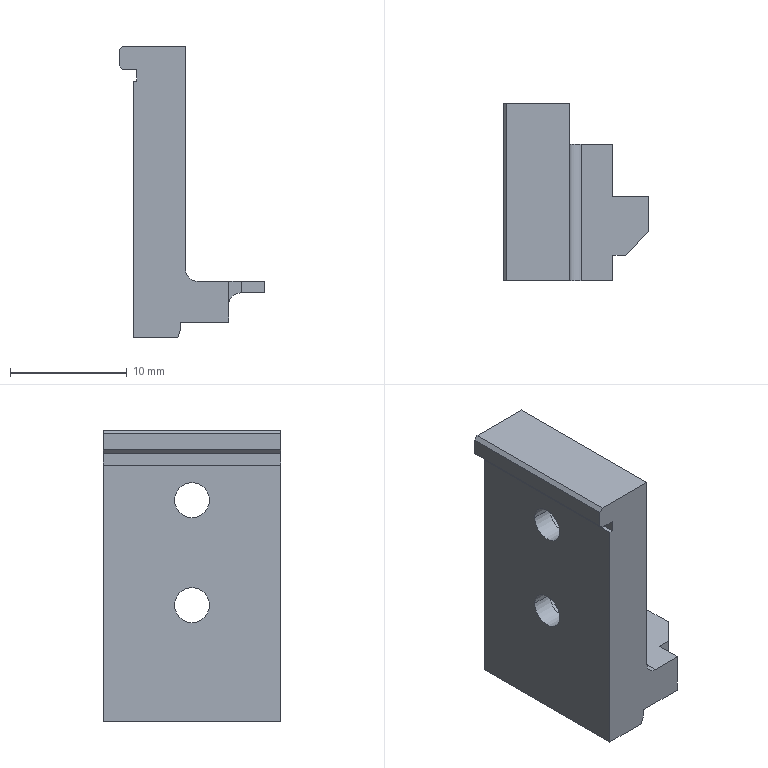Part | NX | 1 solid | 35 faces | box 12.5 x 15.2 x 25 mm | volume 1768 mm3 | plane 25 | cylinder 10 | commonest cylinder face diameters 3 x4 5 x4 2 x2
STEP:
#1=CARTESIAN_POINT('',(-1.77,0.,-1.43));
#2=VERTEX_POINT('',#1);
#3=CARTESIAN_POINT('',(-2.025,0.,-2.13));
#4=VERTEX_POINT('',#3);
#5=CARTESIAN_POINT('',(-1.25,0.,0.));
#6=DIRECTION('',(-0.342,0.,-0.9397));
#7=VECTOR('',#6,1000.);
#8=LINE('',#5,#7);
#9=EDGE_CURVE('',#2,#4,#8,.T.);
#10=ORIENTED_EDGE('',*,*,#9,.T.);
#11=CARTESIAN_POINT('',(-5.85,0.,-2.13));
#12=VERTEX_POINT('',#11);
#13=CARTESIAN_POINT('',(0.,0.,-2.13));
#14=DIRECTION('',(1.,0.,0.));
#15=VECTOR('',#14,1000.);
#16=LINE('',#13,#15);
#17=EDGE_CURVE('',#12,#4,#16,.T.);
#18=ORIENTED_EDGE('',*,*,#17,.F.);
#19=CARTESIAN_POINT('',(-5.85,0.,19.87));
#20=VERTEX_POINT('',#19);
#21=CARTESIAN_POINT('',(-5.85,0.,0.));
#22=DIRECTION('',(0.,0.,1.));
#23=VECTOR('',#22,1000.);
#24=LINE('',#21,#23);
#25=EDGE_CURVE('',#12,#20,#24,.T.);
#26=ORIENTED_EDGE('',*,*,#25,.T.);
#27=CARTESIAN_POINT('',(-5.55,0.,19.87));
#28=VERTEX_POINT('',#27);
#29=CARTESIAN_POINT('',(0.,0.,19.87));
#30=DIRECTION('',(1.,0.,0.));
#31=VECTOR('',#30,1000.);
#32=LINE('',#29,#31);
#33=EDGE_CURVE('',#20,#28,#32,.T.);
#34=ORIENTED_EDGE('',*,*,#33,.T.);
#35=CARTESIAN_POINT('',(-5.55,0.,20.87));
#36=VERTEX_POINT('',#35);
#37=CARTESIAN_POINT('',(-5.55,0.,0.));
#38=DIRECTION('',(0.,0.,1.));
#39=VECTOR('',#38,1000.);
#40=LINE('',#37,#39);
#41=EDGE_CURVE('',#28,#36,#40,.T.);
#42=ORIENTED_EDGE('',*,*,#41,.T.);
#43=CARTESIAN_POINT('',(-6.75,0.,20.87));
#44=VERTEX_POINT('',#43);
#45=CARTESIAN_POINT('',(0.,0.,20.87));
#46=DIRECTION('',(-1.,0.,0.));
#47=VECTOR('',#46,1000.);
#48=LINE('',#45,#47);
#49=EDGE_CURVE('',#36,#44,#48,.T.);
#50=ORIENTED_EDGE('',*,*,#49,.T.);
#51=CARTESIAN_POINT('',(-7.05,0.,21.17));
#52=VERTEX_POINT('',#51);
#53=CARTESIAN_POINT('',(14.12,0.,0.));
#54=DIRECTION('',(0.7071,0.,-0.7071));
#55=VECTOR('',#54,1000.);
#56=LINE('',#53,#55);
#57=EDGE_CURVE('',#52,#44,#56,.T.);
#58=ORIENTED_EDGE('',*,*,#57,.F.);
#59=CARTESIAN_POINT('',(-7.05,0.,22.57));
#60=VERTEX_POINT('',#59);
#61=CARTESIAN_POINT('',(-7.05,0.,0.));
#62=DIRECTION('',(0.,0.,1.));
#63=VECTOR('',#62,1000.);
#64=LINE('',#61,#63);
#65=EDGE_CURVE('',#52,#60,#64,.T.);
#66=ORIENTED_EDGE('',*,*,#65,.T.);
#67=CARTESIAN_POINT('',(-6.75,0.,22.87));
#68=VERTEX_POINT('',#67);
#69=CARTESIAN_POINT('',(-29.62,0.,0.));
#70=DIRECTION('',(0.7071,0.,0.7071));
#71=VECTOR('',#70,1000.);
#72=LINE('',#69,#71);
#73=EDGE_CURVE('',#60,#68,#72,.T.);
#74=ORIENTED_EDGE('',*,*,#73,.T.);
#75=CARTESIAN_POINT('',(-1.35,0.,22.87));
#76=VERTEX_POINT('',#75);
#77=CARTESIAN_POINT('',(0.,0.,22.87));
#78=DIRECTION('',(1.,0.,0.));
#79=VECTOR('',#78,1000.);
#80=LINE('',#77,#79);
#81=EDGE_CURVE('',#68,#76,#80,.T.);
#82=ORIENTED_EDGE('',*,*,#81,.T.);
#83=CARTESIAN_POINT('',(-1.35,0.,-0.78));
#84=VERTEX_POINT('',#83);
#85=CARTESIAN_POINT('',(-1.35,0.,0.));
#86=DIRECTION('',(0.,0.,1.));
#87=VECTOR('',#86,1000.);
#88=LINE('',#85,#87);
#89=EDGE_CURVE('',#84,#76,#88,.T.);
#90=ORIENTED_EDGE('',*,*,#89,.F.);
#91=CARTESIAN_POINT('',(-1.77,0.,-0.78));
#92=VERTEX_POINT('',#91);
#93=CARTESIAN_POINT('',(0.,0.,-0.78));
#94=DIRECTION('',(-1.,0.,0.));
#95=VECTOR('',#94,1000.);
#96=LINE('',#93,#95);
#97=EDGE_CURVE('',#84,#92,#96,.T.);
#98=ORIENTED_EDGE('',*,*,#97,.T.);
#99=CARTESIAN_POINT('',(-1.77,0.,0.));
#100=DIRECTION('',(0.,0.,-1.));
#101=VECTOR('',#100,1000.);
#102=LINE('',#99,#101);
#103=EDGE_CURVE('',#92,#2,#102,.T.);
#104=ORIENTED_EDGE('',*,*,#103,.T.);
#105=EDGE_LOOP('',(#10,#18,#26,#34,#42,#50,#58,#66,#74,#82,#90,#98,#104));
#106=FACE_BOUND('',#105,.T.);
#107=CARTESIAN_POINT('',(0.,0.,0.));
#108=DIRECTION('',(0.,-1.,0.));
#109=DIRECTION('',(0.,0.,-1.));
#110=AXIS2_PLACEMENT_3D('',#107,#108,#109);
#111=PLANE('',#110);
#112=ADVANCED_FACE('',(#106),#111,.F.);
#113=CARTESIAN_POINT('',(-1.77,-15.2,-1.43));
#114=VERTEX_POINT('',#113);
#115=CARTESIAN_POINT('',(-1.77,0.,-1.43));
#116=DIRECTION('',(0.,-1.,0.));
#117=VECTOR('',#116,1000.);
#118=LINE('',#115,#117);
#119=EDGE_CURVE('',#2,#114,#118,.T.);
#120=ORIENTED_EDGE('',*,*,#119,.F.);
#121=ORIENTED_EDGE('',*,*,#103,.F.);
#122=CARTESIAN_POINT('',(-1.77,-15.2,-0.78));
#123=VERTEX_POINT('',#122);
#124=CARTESIAN_POINT('',(-1.77,0.,-0.78));
#125=DIRECTION('',(0.,1.,0.));
#126=VECTOR('',#125,1000.);
#127=LINE('',#124,#126);
#128=EDGE_CURVE('',#123,#92,#127,.T.);
#129=ORIENTED_EDGE('',*,*,#128,.F.);
#130=CARTESIAN_POINT('',(-1.77,-15.2,0.));
#131=DIRECTION('',(0.,0.,1.));
#132=VECTOR('',#131,1000.);
#133=LINE('',#130,#132);
#134=EDGE_CURVE('',#114,#123,#133,.T.);
#135=ORIENTED_EDGE('',*,*,#134,.F.);
#136=EDGE_LOOP('',(#120,#121,#129,#135));
#137=FACE_BOUND('',#136,.T.);
#138=CARTESIAN_POINT('',(-1.77,0.,-0.93));
#139=DIRECTION('',(1.,0.,0.));
#140=DIRECTION('',(0.,1.,0.));
#141=AXIS2_PLACEMENT_3D('',#138,#139,#140);
#142=PLANE('',#141);
#143=ADVANCED_FACE('',(#137),#142,.T.);
#144=CARTESIAN_POINT('',(-0.35,-15.2,2.72));
#145=VERTEX_POINT('',#144);
#146=CARTESIAN_POINT('',(2.35,-15.2,2.72));
#147=VERTEX_POINT('',#146);
#148=CARTESIAN_POINT('',(0.,-15.2,2.72));
#149=DIRECTION('',(1.,0.,0.));
#150=VECTOR('',#149,1000.);
#151=LINE('',#148,#150);
#152=EDGE_CURVE('',#145,#147,#151,.T.);
#153=ORIENTED_EDGE('',*,*,#152,.F.);
#154=CARTESIAN_POINT('',(-1.35,-15.2,3.72));
#155=VERTEX_POINT('',#154);
#156=CARTESIAN_POINT('',(-0.35,-15.2,3.72));
#157=DIRECTION('',(0.,1.,0.));
#158=DIRECTION('',(-1.,0.,0.));
#159=AXIS2_PLACEMENT_3D('',#156,#157,#158);
#160=CIRCLE('',#159,1.);
#161=EDGE_CURVE('',#145,#155,#160,.T.);
#162=ORIENTED_EDGE('',*,*,#161,.T.);
#163=CARTESIAN_POINT('',(-1.35,-15.2,22.87));
#164=VERTEX_POINT('',#163);
#165=CARTESIAN_POINT('',(-1.35,-15.2,0.));
#166=DIRECTION('',(0.,0.,-1.));
#167=VECTOR('',#166,1000.);
#168=LINE('',#165,#167);
#169=EDGE_CURVE('',#164,#155,#168,.T.);
#170=ORIENTED_EDGE('',*,*,#169,.F.);
#171=CARTESIAN_POINT('',(-6.75,-15.2,22.87));
#172=VERTEX_POINT('',#171);
#173=CARTESIAN_POINT('',(0.,-15.2,22.87));
#174=DIRECTION('',(-1.,0.,0.));
#175=VECTOR('',#174,1000.);
#176=LINE('',#173,#175);
#177=EDGE_CURVE('',#164,#172,#176,.T.);
#178=ORIENTED_EDGE('',*,*,#177,.T.);
#179=CARTESIAN_POINT('',(-7.05,-15.2,22.57));
#180=VERTEX_POINT('',#179);
#181=CARTESIAN_POINT('',(-29.62,-15.2,0.));
#182=DIRECTION('',(-0.7071,0.,-0.7071));
#183=VECTOR('',#182,1000.);
#184=LINE('',#181,#183);
#185=EDGE_CURVE('',#172,#180,#184,.T.);
#186=ORIENTED_EDGE('',*,*,#185,.T.);
#187=CARTESIAN_POINT('',(-7.05,-15.2,21.17));
#188=VERTEX_POINT('',#187);
#189=CARTESIAN_POINT('',(-7.05,-15.2,0.));
#190=DIRECTION('',(0.,0.,-1.));
#191=VECTOR('',#190,1000.);
#192=LINE('',#189,#191);
#193=EDGE_CURVE('',#180,#188,#192,.T.);
#194=ORIENTED_EDGE('',*,*,#193,.T.);
#195=CARTESIAN_POINT('',(-6.75,-15.2,20.87));
#196=VERTEX_POINT('',#195);
#197=CARTESIAN_POINT('',(14.12,-15.2,0.));
#198=DIRECTION('',(-0.7071,0.,0.7071));
#199=VECTOR('',#198,1000.);
#200=LINE('',#197,#199);
#201=EDGE_CURVE('',#196,#188,#200,.T.);
#202=ORIENTED_EDGE('',*,*,#201,.F.);
#203=CARTESIAN_POINT('',(-5.55,-15.2,20.87));
#204=VERTEX_POINT('',#203);
#205=CARTESIAN_POINT('',(0.,-15.2,20.87));
#206=DIRECTION('',(1.,0.,0.));
#207=VECTOR('',#206,1000.);
#208=LINE('',#205,#207);
#209=EDGE_CURVE('',#196,#204,#208,.T.);
#210=ORIENTED_EDGE('',*,*,#209,.T.);
#211=CARTESIAN_POINT('',(-5.55,-15.2,19.87));
#212=VERTEX_POINT('',#211);
#213=CARTESIAN_POINT('',(-5.55,-15.2,0.));
#214=DIRECTION('',(0.,0.,-1.));
#215=VECTOR('',#214,1000.);
#216=LINE('',#213,#215);
#217=EDGE_CURVE('',#204,#212,#216,.T.);
#218=ORIENTED_EDGE('',*,*,#217,.T.);
#219=CARTESIAN_POINT('',(-5.85,-15.2,19.87));
#220=VERTEX_POINT('',#219);
#221=CARTESIAN_POINT('',(0.,-15.2,19.87));
#222=DIRECTION('',(-1.,0.,0.));
#223=VECTOR('',#222,1000.);
#224=LINE('',#221,#223);
#225=EDGE_CURVE('',#212,#220,#224,.T.);
#226=ORIENTED_EDGE('',*,*,#225,.T.);
#227=CARTESIAN_POINT('',(-5.85,-15.2,-2.13));
#228=VERTEX_POINT('',#227);
#229=CARTESIAN_POINT('',(-5.85,-15.2,0.));
#230=DIRECTION('',(0.,0.,-1.));
#231=VECTOR('',#230,1000.);
#232=LINE('',#229,#231);
#233=EDGE_CURVE('',#220,#228,#232,.T.);
#234=ORIENTED_EDGE('',*,*,#233,.T.);
#235=CARTESIAN_POINT('',(-2.025,-15.2,-2.13));
#236=VERTEX_POINT('',#235);
#237=CARTESIAN_POINT('',(0.,-15.2,-2.13));
#238=DIRECTION('',(-1.,0.,0.));
#239=VECTOR('',#238,1000.);
#240=LINE('',#237,#239);
#241=EDGE_CURVE('',#236,#228,#240,.T.);
#242=ORIENTED_EDGE('',*,*,#241,.F.);
#243=CARTESIAN_POINT('',(-1.25,-15.2,0.));
#244=DIRECTION('',(0.342,0.,0.9397));
#245=VECTOR('',#244,1000.);
#246=LINE('',#243,#245);
#247=EDGE_CURVE('',#236,#114,#246,.T.);
#248=ORIENTED_EDGE('',*,*,#247,.T.);
#249=ORIENTED_EDGE('',*,*,#134,.T.);
#250=CARTESIAN_POINT('',(2.35,-15.2,-0.78));
#251=VERTEX_POINT('',#250);
#252=CARTESIAN_POINT('',(0.,-15.2,-0.78));
#253=DIRECTION('',(1.,0.,0.));
#254=VECTOR('',#253,1000.);
#255=LINE('',#252,#254);
#256=EDGE_CURVE('',#123,#251,#255,.T.);
#257=ORIENTED_EDGE('',*,*,#256,.T.);
#258=CARTESIAN_POINT('',(2.35,-15.2,0.));
#259=DIRECTION('',(0.,0.,1.));
#260=VECTOR('',#259,1000.);
#261=LINE('',#258,#260);
#262=EDGE_CURVE('',#251,#147,#261,.T.);
#263=ORIENTED_EDGE('',*,*,#262,.T.);
#264=EDGE_LOOP('',(#153,#162,#170,#178,#186,#194,#202,#210,#218,#226,#234,#242,#248,#249,#257,#263));
#265=FACE_BOUND('',#264,.T.);
#266=CARTESIAN_POINT('',(-1.35,-15.2,0.));
#267=DIRECTION('',(0.,1.,0.));
#268=DIRECTION('',(1.,0.,0.));
#269=AXIS2_PLACEMENT_3D('',#266,#267,#268);
#270=PLANE('',#269);
#271=ADVANCED_FACE('',(#265),#270,.F.);
#272=CARTESIAN_POINT('',(-4.05,-10.1,7.87));
#273=VERTEX_POINT('',#272);
#274=CARTESIAN_POINT('',(-4.05,-5.1,7.87));
#275=VERTEX_POINT('',#274);
#276=CARTESIAN_POINT('',(-4.05,-7.6,7.87));
#277=DIRECTION('',(1.,0.,0.));
#278=DIRECTION('',(0.,-1.,0.));
#279=AXIS2_PLACEMENT_3D('',#276,#277,#278);
#280=CIRCLE('',#279,2.5);
#281=EDGE_CURVE('',#273,#275,#280,.T.);
#282=ORIENTED_EDGE('',*,*,#281,.T.);
#283=CARTESIAN_POINT('',(-4.05,-7.6,7.87));
#284=DIRECTION('',(1.,0.,0.));
#285=DIRECTION('',(0.,-1.,0.));
#286=AXIS2_PLACEMENT_3D('',#283,#284,#285);
#287=CIRCLE('',#286,2.5);
#288=EDGE_CURVE('',#275,#273,#287,.T.);
#289=ORIENTED_EDGE('',*,*,#288,.T.);
#290=EDGE_LOOP('',(#282,#289));
#291=FACE_BOUND('',#290,.T.);
#292=CARTESIAN_POINT('',(-4.05,-6.1,7.87));
#293=VERTEX_POINT('',#292);
#294=CARTESIAN_POINT('',(-4.05,-9.1,7.87));
#295=VERTEX_POINT('',#294);
#296=CARTESIAN_POINT('',(-4.05,-7.6,7.87));
#297=DIRECTION('',(1.,0.,0.));
#298=DIRECTION('',(0.,-1.,0.));
#299=AXIS2_PLACEMENT_3D('',#296,#297,#298);
#300=CIRCLE('',#299,1.5);
#301=EDGE_CURVE('',#293,#295,#300,.T.);
#302=ORIENTED_EDGE('',*,*,#301,.F.);
#303=CARTESIAN_POINT('',(-4.05,-7.6,7.87));
#304=DIRECTION('',(1.,0.,0.));
#305=DIRECTION('',(0.,-1.,0.));
#306=AXIS2_PLACEMENT_3D('',#303,#304,#305);
#307=CIRCLE('',#306,1.5);
#308=EDGE_CURVE('',#295,#293,#307,.T.);
#309=ORIENTED_EDGE('',*,*,#308,.F.);
#310=EDGE_LOOP('',(#302,#309));
#311=FACE_BOUND('',#310,.T.);
#312=CARTESIAN_POINT('',(-4.05,-7.6,7.87));
#313=DIRECTION('',(-1.,0.,0.));
#314=DIRECTION('',(0.,0.,1.));
#315=AXIS2_PLACEMENT_3D('',#312,#313,#314);
#316=PLANE('',#315);
#317=ADVANCED_FACE('',(#291,#311),#316,.F.);
#318=ORIENTED_EDGE('',*,*,#241,.T.);
#319=CARTESIAN_POINT('',(-5.85,0.,-2.13));
#320=DIRECTION('',(0.,1.,0.));
#321=VECTOR('',#320,1000.);
#322=LINE('',#319,#321);
#323=EDGE_CURVE('',#228,#12,#322,.T.);
#324=ORIENTED_EDGE('',*,*,#323,.T.);
#325=ORIENTED_EDGE('',*,*,#17,.T.);
#326=CARTESIAN_POINT('',(-2.025,0.,-2.13));
#327=DIRECTION('',(0.,-1.,0.));
#328=VECTOR('',#327,1000.);
#329=LINE('',#326,#328);
#330=EDGE_CURVE('',#4,#236,#329,.T.);
#331=ORIENTED_EDGE('',*,*,#330,.T.);
#332=EDGE_LOOP('',(#318,#324,#325,#331));
#333=FACE_BOUND('',#332,.T.);
#334=CARTESIAN_POINT('',(0.,0.,-2.13));
#335=DIRECTION('',(0.,0.,1.));
#336=DIRECTION('',(1.,0.,0.));
#337=AXIS2_PLACEMENT_3D('',#334,#335,#336);
#338=PLANE('',#337);
#339=ADVANCED_FACE('',(#333),#338,.F.);
#340=ORIENTED_EDGE('',*,*,#9,.F.);
#341=ORIENTED_EDGE('',*,*,#119,.T.);
#342=ORIENTED_EDGE('',*,*,#247,.F.);
#343=ORIENTED_EDGE('',*,*,#330,.F.);
#344=EDGE_LOOP('',(#340,#341,#342,#343));
#345=FACE_BOUND('',#344,.T.);
#346=CARTESIAN_POINT('',(-2.025,-15.2,-2.13));
#347=DIRECTION('',(0.9397,0.,-0.342));
#348=DIRECTION('',(0.,-1.,0.));
#349=AXIS2_PLACEMENT_3D('',#346,#347,#348);
#350=PLANE('',#349);
#351=ADVANCED_FACE('',(#345),#350,.T.);
#352=CARTESIAN_POINT('',(-5.85,0.,19.87));
#353=DIRECTION('',(0.,-1.,0.));
#354=VECTOR('',#353,1000.);
#355=LINE('',#352,#354);
#356=EDGE_CURVE('',#20,#220,#355,.T.);
#357=ORIENTED_EDGE('',*,*,#356,.T.);
#358=ORIENTED_EDGE('',*,*,#225,.F.);
#359=CARTESIAN_POINT('',(-5.55,0.,19.87));
#360=DIRECTION('',(0.,-1.,0.));
#361=VECTOR('',#360,1000.);
#362=LINE('',#359,#361);
#363=EDGE_CURVE('',#28,#212,#362,.T.);
#364=ORIENTED_EDGE('',*,*,#363,.F.);
#365=ORIENTED_EDGE('',*,*,#33,.F.);
#366=EDGE_LOOP('',(#357,#358,#364,#365));
#367=FACE_BOUND('',#366,.T.);
#368=CARTESIAN_POINT('',(-4.85,0.,19.87));
#369=DIRECTION('',(0.,0.,1.));
#370=DIRECTION('',(1.,0.,0.));
#371=AXIS2_PLACEMENT_3D('',#368,#369,#370);
#372=PLANE('',#371);
#373=ADVANCED_FACE('',(#367),#372,.T.);
#374=ORIENTED_EDGE('',*,*,#363,.T.);
#375=ORIENTED_EDGE('',*,*,#217,.F.);
#376=CARTESIAN_POINT('',(-5.55,0.,20.87));
#377=DIRECTION('',(0.,-1.,0.));
#378=VECTOR('',#377,1000.);
#379=LINE('',#376,#378);
#380=EDGE_CURVE('',#36,#204,#379,.T.);
#381=ORIENTED_EDGE('',*,*,#380,.F.);
#382=ORIENTED_EDGE('',*,*,#41,.F.);
#383=EDGE_LOOP('',(#374,#375,#381,#382));
#384=FACE_BOUND('',#383,.T.);
#385=CARTESIAN_POINT('',(-5.55,0.,19.87));
#386=DIRECTION('',(-1.,0.,0.));
#387=DIRECTION('',(0.,0.,1.));
#388=AXIS2_PLACEMENT_3D('',#385,#386,#387);
#389=PLANE('',#388);
#390=ADVANCED_FACE('',(#384),#389,.T.);
#391=CARTESIAN_POINT('',(-6.75,0.,20.87));
#392=DIRECTION('',(0.,1.,0.));
#393=VECTOR('',#392,1000.);
#394=LINE('',#391,#393);
#395=EDGE_CURVE('',#196,#44,#394,.T.);
#396=ORIENTED_EDGE('',*,*,#395,.T.);
#397=ORIENTED_EDGE('',*,*,#49,.F.);
#398=ORIENTED_EDGE('',*,*,#380,.T.);
#399=ORIENTED_EDGE('',*,*,#209,.F.);
#400=EDGE_LOOP('',(#396,#397,#398,#399));
#401=FACE_BOUND('',#400,.T.);
#402=CARTESIAN_POINT('',(-4.85,0.,20.87));
#403=DIRECTION('',(0.,0.,-1.));
#404=DIRECTION('',(0.,-1.,0.));
#405=AXIS2_PLACEMENT_3D('',#402,#403,#404);
#406=PLANE('',#405);
#407=ADVANCED_FACE('',(#401),#406,.T.);
#408=CARTESIAN_POINT('',(-7.05,0.,22.57));
#409=DIRECTION('',(0.,-1.,0.));
#410=VECTOR('',#409,1000.);
#411=LINE('',#408,#410);
#412=EDGE_CURVE('',#60,#180,#411,.T.);
#413=ORIENTED_EDGE('',*,*,#412,.F.);
#414=ORIENTED_EDGE('',*,*,#65,.F.);
#415=CARTESIAN_POINT('',(-7.05,0.,21.17));
#416=DIRECTION('',(0.,-1.,0.));
#417=VECTOR('',#416,1000.);
#418=LINE('',#415,#417);
#419=EDGE_CURVE('',#52,#188,#418,.T.);
#420=ORIENTED_EDGE('',*,*,#419,.T.);
#421=ORIENTED_EDGE('',*,*,#193,.F.);
#422=EDGE_LOOP('',(#413,#414,#420,#421));
#423=FACE_BOUND('',#422,.T.);
#424=CARTESIAN_POINT('',(-7.05,0.,20.87));
#425=DIRECTION('',(-1.,0.,0.));
#426=DIRECTION('',(0.,0.,1.));
#427=AXIS2_PLACEMENT_3D('',#424,#425,#426);
#428=PLANE('',#427);
#429=ADVANCED_FACE('',(#423),#428,.T.);
#430=CARTESIAN_POINT('',(-6.75,0.,22.87));
#431=DIRECTION('',(0.,1.,0.));
#432=VECTOR('',#431,1000.);
#433=LINE('',#430,#432);
#434=EDGE_CURVE('',#172,#68,#433,.T.);
#435=ORIENTED_EDGE('',*,*,#434,.F.);
#436=ORIENTED_EDGE('',*,*,#177,.F.);
#437=CARTESIAN_POINT('',(-1.35,0.,22.87));
#438=DIRECTION('',(0.,-1.,0.));
#439=VECTOR('',#438,1000.);
#440=LINE('',#437,#439);
#441=EDGE_CURVE('',#76,#164,#440,.T.);
#442=ORIENTED_EDGE('',*,*,#441,.F.);
#443=ORIENTED_EDGE('',*,*,#81,.F.);
#444=EDGE_LOOP('',(#435,#436,#442,#443));
#445=FACE_BOUND('',#444,.T.);
#446=CARTESIAN_POINT('',(-6.05,0.,22.87));
#447=DIRECTION('',(0.,0.,1.));
#448=DIRECTION('',(1.,0.,0.));
#449=AXIS2_PLACEMENT_3D('',#446,#447,#448);
#450=PLANE('',#449);
#451=ADVANCED_FACE('',(#445),#450,.T.);
#452=ORIENTED_EDGE('',*,*,#169,.T.);
#453=CARTESIAN_POINT('',(-1.35,-3.5,3.72));
#454=VERTEX_POINT('',#453);
#455=CARTESIAN_POINT('',(-1.35,-15.285,3.72));
#456=DIRECTION('',(0.,1.,0.));
#457=VECTOR('',#456,1000.);
#458=LINE('',#455,#457);
#459=EDGE_CURVE('',#155,#454,#458,.T.);
#460=ORIENTED_EDGE('',*,*,#459,.T.);
#461=CARTESIAN_POINT('',(-1.35,-3.5,-0.78));
#462=VERTEX_POINT('',#461);
#463=CARTESIAN_POINT('',(-1.35,-3.5,0.));
#464=DIRECTION('',(0.,0.,-1.));
#465=VECTOR('',#464,1000.);
#466=LINE('',#463,#465);
#467=EDGE_CURVE('',#454,#462,#466,.T.);
#468=ORIENTED_EDGE('',*,*,#467,.T.);
#469=CARTESIAN_POINT('',(-1.35,0.,-0.78));
#470=DIRECTION('',(0.,1.,0.));
#471=VECTOR('',#470,1000.);
#472=LINE('',#469,#471);
#473=EDGE_CURVE('',#462,#84,#472,.T.);
#474=ORIENTED_EDGE('',*,*,#473,.T.);
#475=ORIENTED_EDGE('',*,*,#89,.T.);
#476=ORIENTED_EDGE('',*,*,#441,.T.);
#477=EDGE_LOOP('',(#452,#460,#468,#474,#475,#476));
#478=FACE_BOUND('',#477,.T.);
#479=CARTESIAN_POINT('',(-1.35,-5.1,16.87));
#480=VERTEX_POINT('',#479);
#481=CARTESIAN_POINT('',(-1.35,-10.1,16.87));
#482=VERTEX_POINT('',#481);
#483=CARTESIAN_POINT('',(-1.35,-7.6,16.87));
#484=DIRECTION('',(1.,0.,0.));
#485=DIRECTION('',(0.,-1.,0.));
#486=AXIS2_PLACEMENT_3D('',#483,#484,#485);
#487=CIRCLE('',#486,2.5);
#488=EDGE_CURVE('',#480,#482,#487,.T.);
#489=ORIENTED_EDGE('',*,*,#488,.F.);
#490=CARTESIAN_POINT('',(-1.35,-7.6,16.87));
#491=DIRECTION('',(1.,0.,0.));
#492=DIRECTION('',(0.,-1.,0.));
#493=AXIS2_PLACEMENT_3D('',#490,#491,#492);
#494=CIRCLE('',#493,2.5);
#495=EDGE_CURVE('',#482,#480,#494,.T.);
#496=ORIENTED_EDGE('',*,*,#495,.F.);
#497=EDGE_LOOP('',(#489,#496));
#498=FACE_BOUND('',#497,.T.);
#499=CARTESIAN_POINT('',(-1.35,-10.1,7.87));
#500=VERTEX_POINT('',#499);
#501=CARTESIAN_POINT('',(-1.35,-5.1,7.87));
#502=VERTEX_POINT('',#501);
#503=CARTESIAN_POINT('',(-1.35,-7.6,7.87));
#504=DIRECTION('',(1.,0.,0.));
#505=DIRECTION('',(0.,-1.,0.));
#506=AXIS2_PLACEMENT_3D('',#503,#504,#505);
#507=CIRCLE('',#506,2.5);
#508=EDGE_CURVE('',#500,#502,#507,.T.);
#509=ORIENTED_EDGE('',*,*,#508,.F.);
#510=CARTESIAN_POINT('',(-1.35,-7.6,7.87));
#511=DIRECTION('',(1.,0.,0.));
#512=DIRECTION('',(0.,-1.,0.));
#513=AXIS2_PLACEMENT_3D('',#510,#511,#512);
#514=CIRCLE('',#513,2.5);
#515=EDGE_CURVE('',#502,#500,#514,.T.);
#516=ORIENTED_EDGE('',*,*,#515,.F.);
#517=EDGE_LOOP('',(#509,#516));
#518=FACE_BOUND('',#517,.T.);
#519=CARTESIAN_POINT('',(-1.35,0.,-1.13));
#520=DIRECTION('',(-1.,0.,0.));
#521=DIRECTION('',(0.,0.,1.));
#522=AXIS2_PLACEMENT_3D('',#519,#520,#521);
#523=PLANE('',#522);
#524=ADVANCED_FACE('',(#478,#498,#518),#523,.F.);
#525=ORIENTED_EDGE('',*,*,#459,.F.);
#526=ORIENTED_EDGE('',*,*,#161,.F.);
#527=CARTESIAN_POINT('',(-0.35,-3.5,2.72));
#528=VERTEX_POINT('',#527);
#529=CARTESIAN_POINT('',(-0.35,-15.2,2.72));
#530=DIRECTION('',(0.,1.,0.));
#531=VECTOR('',#530,1000.);
#532=LINE('',#529,#531);
#533=EDGE_CURVE('',#145,#528,#532,.T.);
#534=ORIENTED_EDGE('',*,*,#533,.T.);
#535=CARTESIAN_POINT('',(-0.35,-3.5,3.72));
#536=DIRECTION('',(0.,1.,0.));
#537=DIRECTION('',(-1.,0.,0.));
#538=AXIS2_PLACEMENT_3D('',#535,#536,#537);
#539=CIRCLE('',#538,1.);
#540=EDGE_CURVE('',#528,#454,#539,.T.);
#541=ORIENTED_EDGE('',*,*,#540,.T.);
#542=EDGE_LOOP('',(#525,#526,#534,#541));
#543=FACE_BOUND('',#542,.T.);
#544=CARTESIAN_POINT('',(-0.35,-15.285,3.72));
#545=DIRECTION('',(0.,1.,0.));
#546=DIRECTION('',(-1.,0.,0.));
#547=AXIS2_PLACEMENT_3D('',#544,#545,#546);
#548=CYLINDRICAL_SURFACE('',#547,1.);
#549=ADVANCED_FACE('',(#543),#548,.F.);
#550=CARTESIAN_POINT('',(2.35,-3.5,2.72));
#551=VERTEX_POINT('',#550);
#552=CARTESIAN_POINT('',(2.35,-3.5,-0.78));
#553=VERTEX_POINT('',#552);
#554=CARTESIAN_POINT('',(2.35,-3.5,0.));
#555=DIRECTION('',(0.,0.,-1.));
#556=VECTOR('',#555,1000.);
#557=LINE('',#554,#556);
#558=EDGE_CURVE('',#551,#553,#557,.T.);
#559=ORIENTED_EDGE('',*,*,#558,.T.);
#560=CARTESIAN_POINT('',(0.,-3.5,-0.78));
#561=DIRECTION('',(-1.,0.,0.));
#562=VECTOR('',#561,1000.);
#563=LINE('',#560,#562);
#564=EDGE_CURVE('',#553,#462,#563,.T.);
#565=ORIENTED_EDGE('',*,*,#564,.T.);
#566=ORIENTED_EDGE('',*,*,#467,.F.);
#567=ORIENTED_EDGE('',*,*,#540,.F.);
#568=CARTESIAN_POINT('',(0.,-3.5,2.72));
#569=DIRECTION('',(1.,0.,0.));
#570=VECTOR('',#569,1000.);
#571=LINE('',#568,#570);
#572=EDGE_CURVE('',#528,#551,#571,.T.);
#573=ORIENTED_EDGE('',*,*,#572,.T.);
#574=EDGE_LOOP('',(#559,#565,#566,#567,#573));
#575=FACE_BOUND('',#574,.T.);
#576=CARTESIAN_POINT('',(-1.77,-3.5,-0.83));
#577=DIRECTION('',(0.,-1.,0.));
#578=DIRECTION('',(0.,0.,-1.));
#579=AXIS2_PLACEMENT_3D('',#576,#577,#578);
#580=PLANE('',#579);
#581=ADVANCED_FACE('',(#575),#580,.F.);
#582=CARTESIAN_POINT('',(3.45,-13.,1.72));
#583=VERTEX_POINT('',#582);
#584=CARTESIAN_POINT('',(3.35,-13.,1.72));
#585=VERTEX_POINT('',#584);
#586=CARTESIAN_POINT('',(0.,-13.,1.72));
#587=DIRECTION('',(-1.,0.,0.));
#588=VECTOR('',#587,1000.);
#589=LINE('',#586,#588);
#590=EDGE_CURVE('',#583,#585,#589,.T.);
#591=ORIENTED_EDGE('',*,*,#590,.T.);
#592=CARTESIAN_POINT('',(3.35,-8.,1.72));
#593=VERTEX_POINT('',#592);
#594=CARTESIAN_POINT('',(3.35,0.,1.72));
#595=DIRECTION('',(0.,-1.,0.));
#596=VECTOR('',#595,1000.);
#597=LINE('',#594,#596);
#598=EDGE_CURVE('',#593,#585,#597,.T.);
#599=ORIENTED_EDGE('',*,*,#598,.F.);
#600=CARTESIAN_POINT('',(5.45,-8.,1.72));
#601=VERTEX_POINT('',#600);
#602=CARTESIAN_POINT('',(0.,-8.,1.72));
#603=DIRECTION('',(-1.,0.,0.));
#604=VECTOR('',#603,1000.);
#605=LINE('',#602,#604);
#606=EDGE_CURVE('',#601,#593,#605,.T.);
#607=ORIENTED_EDGE('',*,*,#606,.F.);
#608=CARTESIAN_POINT('',(5.45,-11.,1.72));
#609=VERTEX_POINT('',#608);
#610=CARTESIAN_POINT('',(5.45,0.,1.72));
#611=DIRECTION('',(0.,1.,0.));
#612=VECTOR('',#611,1000.);
#613=LINE('',#610,#612);
#614=EDGE_CURVE('',#609,#601,#613,.T.);
#615=ORIENTED_EDGE('',*,*,#614,.F.);
#616=CARTESIAN_POINT('',(16.45,0.,1.72));
#617=DIRECTION('',(-0.7071,-0.7071,0.));
#618=VECTOR('',#617,1000.);
#619=LINE('',#616,#618);
#620=EDGE_CURVE('',#609,#583,#619,.T.);
#621=ORIENTED_EDGE('',*,*,#620,.T.);
#622=EDGE_LOOP('',(#591,#599,#607,#615,#621));
#623=FACE_BOUND('',#622,.T.);
#624=CARTESIAN_POINT('',(5.45,-6.5,1.72));
#625=DIRECTION('',(0.,0.,1.));
#626=DIRECTION('',(1.,0.,0.));
#627=AXIS2_PLACEMENT_3D('',#624,#625,#626);
#628=PLANE('',#627);
#629=ADVANCED_FACE('',(#623),#628,.F.);
#630=ORIENTED_EDGE('',*,*,#508,.T.);
#631=CARTESIAN_POINT('',(-7.072,-5.1,7.87));
#632=DIRECTION('',(1.,0.,0.));
#633=VECTOR('',#632,1000.);
#634=LINE('',#631,#633);
#635=EDGE_CURVE('',#502,#275,#634,.F.);
#636=ORIENTED_EDGE('',*,*,#635,.T.);
#637=ORIENTED_EDGE('',*,*,#281,.F.);
#638=CARTESIAN_POINT('',(-7.072,-10.1,7.87));
#639=DIRECTION('',(1.,0.,0.));
#640=VECTOR('',#639,1000.);
#641=LINE('',#638,#640);
#642=EDGE_CURVE('',#500,#273,#641,.F.);
#643=ORIENTED_EDGE('',*,*,#642,.F.);
#644=EDGE_LOOP('',(#630,#636,#637,#643));
#645=FACE_BOUND('',#644,.T.);
#646=CARTESIAN_POINT('',(-7.072,-7.6,7.87));
#647=DIRECTION('',(1.,0.,0.));
#648=DIRECTION('',(0.,-1.,0.));
#649=AXIS2_PLACEMENT_3D('',#646,#647,#648);
#650=CYLINDRICAL_SURFACE('',#649,2.5);
#651=ADVANCED_FACE('',(#645),#650,.F.);
#652=ORIENTED_EDGE('',*,*,#572,.F.);
#653=ORIENTED_EDGE('',*,*,#533,.F.);
#654=ORIENTED_EDGE('',*,*,#152,.T.);
#655=CARTESIAN_POINT('',(2.35,-13.,2.72));
#656=VERTEX_POINT('',#655);
#657=CARTESIAN_POINT('',(2.35,0.,2.72));
#658=DIRECTION('',(0.,1.,0.));
#659=VECTOR('',#658,1000.);
#660=LINE('',#657,#659);
#661=EDGE_CURVE('',#147,#656,#660,.T.);
#662=ORIENTED_EDGE('',*,*,#661,.T.);
#663=CARTESIAN_POINT('',(3.45,-13.,2.72));
#664=VERTEX_POINT('',#663);
#665=CARTESIAN_POINT('',(0.,-13.,2.72));
#666=DIRECTION('',(1.,0.,0.));
#667=VECTOR('',#666,1000.);
#668=LINE('',#665,#667);
#669=EDGE_CURVE('',#656,#664,#668,.T.);
#670=ORIENTED_EDGE('',*,*,#669,.T.);
#671=CARTESIAN_POINT('',(5.45,-11.,2.72));
#672=VERTEX_POINT('',#671);
#673=CARTESIAN_POINT('',(16.45,0.,2.72));
#674=DIRECTION('',(-0.7071,-0.7071,0.));
#675=VECTOR('',#674,1000.);
#676=LINE('',#673,#675);
#677=EDGE_CURVE('',#672,#664,#676,.T.);
#678=ORIENTED_EDGE('',*,*,#677,.F.);
#679=CARTESIAN_POINT('',(5.45,-8.,2.72));
#680=VERTEX_POINT('',#679);
#681=CARTESIAN_POINT('',(5.45,0.,2.72));
#682=DIRECTION('',(0.,1.,0.));
#683=VECTOR('',#682,1000.);
#684=LINE('',#681,#683);
#685=EDGE_CURVE('',#672,#680,#684,.T.);
#686=ORIENTED_EDGE('',*,*,#685,.T.);
#687=CARTESIAN_POINT('',(2.35,-8.,2.72));
#688=VERTEX_POINT('',#687);
#689=CARTESIAN_POINT('',(0.,-8.,2.72));
#690=DIRECTION('',(-1.,0.,0.));
#691=VECTOR('',#690,1000.);
#692=LINE('',#689,#691);
#693=EDGE_CURVE('',#680,#688,#692,.T.);
#694=ORIENTED_EDGE('',*,*,#693,.T.);
#695=CARTESIAN_POINT('',(2.35,0.,2.72));
#696=DIRECTION('',(0.,1.,0.));
#697=VECTOR('',#696,1000.);
#698=LINE('',#695,#697);
#699=EDGE_CURVE('',#688,#551,#698,.T.);
#700=ORIENTED_EDGE('',*,*,#699,.T.);
#701=EDGE_LOOP('',(#652,#653,#654,#662,#670,#678,#686,#694,#700));
#702=FACE_BOUND('',#701,.T.);
#703=CARTESIAN_POINT('',(-1.35,-15.2,2.72));
#704=DIRECTION('',(0.,0.,-1.));
#705=DIRECTION('',(0.,-1.,0.));
#706=AXIS2_PLACEMENT_3D('',#703,#704,#705);
#707=PLANE('',#706);
#708=ADVANCED_FACE('',(#702),#707,.F.);
#709=CARTESIAN_POINT('',(2.35,-13.,0.72));
#710=VERTEX_POINT('',#709);
#711=CARTESIAN_POINT('',(2.35,-13.,0.));
#712=DIRECTION('',(0.,0.,-1.));
#713=VECTOR('',#712,1000.);
#714=LINE('',#711,#713);
#715=EDGE_CURVE('',#656,#710,#714,.T.);
#716=ORIENTED_EDGE('',*,*,#715,.T.);
#717=CARTESIAN_POINT('',(3.35,-13.,0.72));
#718=DIRECTION('',(0.,-1.,0.));
#719=DIRECTION('',(-1.,0.,0.));
#720=AXIS2_PLACEMENT_3D('',#717,#718,#719);
#721=CIRCLE('',#720,1.);
#722=EDGE_CURVE('',#585,#710,#721,.T.);
#723=ORIENTED_EDGE('',*,*,#722,.F.);
#724=ORIENTED_EDGE('',*,*,#590,.F.);
#725=CARTESIAN_POINT('',(3.45,-13.,0.));
#726=DIRECTION('',(0.,0.,-1.));
#727=VECTOR('',#726,1000.);
#728=LINE('',#725,#727);
#729=EDGE_CURVE('',#664,#583,#728,.T.);
#730=ORIENTED_EDGE('',*,*,#729,.F.);
#731=ORIENTED_EDGE('',*,*,#669,.F.);
#732=EDGE_LOOP('',(#716,#723,#724,#730,#731));
#733=FACE_BOUND('',#732,.T.);
#734=CARTESIAN_POINT('',(2.35,-13.,-0.78));
#735=DIRECTION('',(0.,-1.,0.));
#736=DIRECTION('',(0.,0.,-1.));
#737=AXIS2_PLACEMENT_3D('',#734,#735,#736);
#738=PLANE('',#737);
#739=ADVANCED_FACE('',(#733),#738,.T.);
#740=CARTESIAN_POINT('',(2.35,-8.,0.72));
#741=VERTEX_POINT('',#740);
#742=CARTESIAN_POINT('',(2.35,0.,0.72));
#743=DIRECTION('',(0.,-1.,0.));
#744=VECTOR('',#743,1000.);
#745=LINE('',#742,#744);
#746=EDGE_CURVE('',#741,#710,#745,.T.);
#747=ORIENTED_EDGE('',*,*,#746,.F.);
#748=CARTESIAN_POINT('',(3.35,-8.,0.72));
#749=DIRECTION('',(0.,-1.,0.));
#750=DIRECTION('',(-1.,0.,0.));
#751=AXIS2_PLACEMENT_3D('',#748,#749,#750);
#752=CIRCLE('',#751,1.);
#753=EDGE_CURVE('',#593,#741,#752,.T.);
#754=ORIENTED_EDGE('',*,*,#753,.F.);
#755=ORIENTED_EDGE('',*,*,#598,.T.);
#756=ORIENTED_EDGE('',*,*,#722,.T.);
#757=EDGE_LOOP('',(#747,#754,#755,#756));
#758=FACE_BOUND('',#757,.T.);
#759=CARTESIAN_POINT('',(3.35,0.,0.72));
#760=DIRECTION('',(0.,-1.,0.));
#761=DIRECTION('',(-1.,0.,0.));
#762=AXIS2_PLACEMENT_3D('',#759,#760,#761);
#763=CYLINDRICAL_SURFACE('',#762,1.);
#764=ADVANCED_FACE('',(#758),#763,.F.);
#765=CARTESIAN_POINT('',(5.45,-11.,0.));
#766=DIRECTION('',(0.,0.,-1.));
#767=VECTOR('',#766,1000.);
#768=LINE('',#765,#767);
#769=EDGE_CURVE('',#672,#609,#768,.T.);
#770=ORIENTED_EDGE('',*,*,#769,.F.);
#771=ORIENTED_EDGE('',*,*,#677,.T.);
#772=ORIENTED_EDGE('',*,*,#729,.T.);
#773=ORIENTED_EDGE('',*,*,#620,.F.);
#774=EDGE_LOOP('',(#770,#771,#772,#773));
#775=FACE_BOUND('',#774,.T.);
#776=CARTESIAN_POINT('',(4.45,-12.,2.22));
#777=DIRECTION('',(-0.7071,0.7071,0.));
#778=DIRECTION('',(0.,0.,1.));
#779=AXIS2_PLACEMENT_3D('',#776,#777,#778);
#780=PLANE('',#779);
#781=ADVANCED_FACE('',(#775),#780,.F.);
#782=ORIENTED_EDGE('',*,*,#488,.T.);
#783=CARTESIAN_POINT('',(-4.05,-10.1,16.87));
#784=VERTEX_POINT('',#783);
#785=CARTESIAN_POINT('',(-7.072,-10.1,16.87));
#786=DIRECTION('',(1.,0.,0.));
#787=VECTOR('',#786,1000.);
#788=LINE('',#785,#787);
#789=EDGE_CURVE('',#482,#784,#788,.F.);
#790=ORIENTED_EDGE('',*,*,#789,.T.);
#791=CARTESIAN_POINT('',(-4.05,-5.1,16.87));
#792=VERTEX_POINT('',#791);
#793=CARTESIAN_POINT('',(-4.05,-7.6,16.87));
#794=DIRECTION('',(1.,0.,0.));
#795=DIRECTION('',(0.,-1.,0.));
#796=AXIS2_PLACEMENT_3D('',#793,#794,#795);
#797=CIRCLE('',#796,2.5);
#798=EDGE_CURVE('',#792,#784,#797,.T.);
#799=ORIENTED_EDGE('',*,*,#798,.F.);
#800=CARTESIAN_POINT('',(-7.072,-5.1,16.87));
#801=DIRECTION('',(1.,0.,0.));
#802=VECTOR('',#801,1000.);
#803=LINE('',#800,#802);
#804=EDGE_CURVE('',#480,#792,#803,.F.);
#805=ORIENTED_EDGE('',*,*,#804,.F.);
#806=EDGE_LOOP('',(#782,#790,#799,#805));
#807=FACE_BOUND('',#806,.T.);
#808=CARTESIAN_POINT('',(-7.072,-7.6,16.87));
#809=DIRECTION('',(1.,0.,0.));
#810=DIRECTION('',(0.,-1.,0.));
#811=AXIS2_PLACEMENT_3D('',#808,#809,#810);
#812=CYLINDRICAL_SURFACE('',#811,2.5);
#813=ADVANCED_FACE('',(#807),#812,.F.);
#814=ORIENTED_EDGE('',*,*,#323,.F.);
#815=ORIENTED_EDGE('',*,*,#233,.F.);
#816=ORIENTED_EDGE('',*,*,#356,.F.);
#817=ORIENTED_EDGE('',*,*,#25,.F.);
#818=EDGE_LOOP('',(#814,#815,#816,#817));
#819=FACE_BOUND('',#818,.T.);
#820=CARTESIAN_POINT('',(-5.85,-9.1,16.87));
#821=VERTEX_POINT('',#820);
#822=CARTESIAN_POINT('',(-5.85,-6.1,16.87));
#823=VERTEX_POINT('',#822);
#824=CARTESIAN_POINT('',(-5.85,-7.6,16.87));
#825=DIRECTION('',(1.,0.,0.));
#826=DIRECTION('',(0.,-1.,0.));
#827=AXIS2_PLACEMENT_3D('',#824,#825,#826);
#828=CIRCLE('',#827,1.5);
#829=EDGE_CURVE('',#821,#823,#828,.T.);
#830=ORIENTED_EDGE('',*,*,#829,.T.);
#831=CARTESIAN_POINT('',(-5.85,-7.6,16.87));
#832=DIRECTION('',(1.,0.,0.));
#833=DIRECTION('',(0.,-1.,0.));
#834=AXIS2_PLACEMENT_3D('',#831,#832,#833);
#835=CIRCLE('',#834,1.5);
#836=EDGE_CURVE('',#823,#821,#835,.T.);
#837=ORIENTED_EDGE('',*,*,#836,.T.);
#838=EDGE_LOOP('',(#830,#837));
#839=FACE_BOUND('',#838,.T.);
#840=CARTESIAN_POINT('',(-5.85,-9.1,7.87));
#841=VERTEX_POINT('',#840);
#842=CARTESIAN_POINT('',(-5.85,-6.1,7.87));
#843=VERTEX_POINT('',#842);
#844=CARTESIAN_POINT('',(-5.85,-7.6,7.87));
#845=DIRECTION('',(1.,0.,0.));
#846=DIRECTION('',(0.,-1.,0.));
#847=AXIS2_PLACEMENT_3D('',#844,#845,#846);
#848=CIRCLE('',#847,1.5);
#849=EDGE_CURVE('',#841,#843,#848,.T.);
#850=ORIENTED_EDGE('',*,*,#849,.T.);
#851=CARTESIAN_POINT('',(-5.85,-7.6,7.87));
#852=DIRECTION('',(1.,0.,0.));
#853=DIRECTION('',(0.,-1.,0.));
#854=AXIS2_PLACEMENT_3D('',#851,#852,#853);
#855=CIRCLE('',#854,1.5);
#856=EDGE_CURVE('',#843,#841,#855,.T.);
#857=ORIENTED_EDGE('',*,*,#856,.T.);
#858=EDGE_LOOP('',(#850,#857));
#859=FACE_BOUND('',#858,.T.);
#860=CARTESIAN_POINT('',(-5.85,0.,-1.13));
#861=DIRECTION('',(-1.,0.,0.));
#862=DIRECTION('',(0.,0.,1.));
#863=AXIS2_PLACEMENT_3D('',#860,#861,#862);
#864=PLANE('',#863);
#865=ADVANCED_FACE('',(#819,#839,#859),#864,.T.);
#866=CARTESIAN_POINT('',(-4.05,-7.6,16.87));
#867=DIRECTION('',(1.,0.,0.));
#868=DIRECTION('',(0.,-1.,0.));
#869=AXIS2_PLACEMENT_3D('',#866,#867,#868);
#870=CIRCLE('',#869,2.5);
#871=EDGE_CURVE('',#784,#792,#870,.T.);
#872=ORIENTED_EDGE('',*,*,#871,.T.);
#873=ORIENTED_EDGE('',*,*,#798,.T.);
#874=EDGE_LOOP('',(#872,#873));
#875=FACE_BOUND('',#874,.T.);
#876=CARTESIAN_POINT('',(-4.05,-9.1,16.87));
#877=VERTEX_POINT('',#876);
#878=CARTESIAN_POINT('',(-4.05,-6.1,16.87));
#879=VERTEX_POINT('',#878);
#880=CARTESIAN_POINT('',(-4.05,-7.6,16.87));
#881=DIRECTION('',(1.,0.,0.));
#882=DIRECTION('',(0.,-1.,0.));
#883=AXIS2_PLACEMENT_3D('',#880,#881,#882);
#884=CIRCLE('',#883,1.5);
#885=EDGE_CURVE('',#877,#879,#884,.T.);
#886=ORIENTED_EDGE('',*,*,#885,.F.);
#887=CARTESIAN_POINT('',(-4.05,-7.6,16.87));
#888=DIRECTION('',(1.,0.,0.));
#889=DIRECTION('',(0.,-1.,0.));
#890=AXIS2_PLACEMENT_3D('',#887,#888,#889);
#891=CIRCLE('',#890,1.5);
#892=EDGE_CURVE('',#879,#877,#891,.T.);
#893=ORIENTED_EDGE('',*,*,#892,.F.);
#894=EDGE_LOOP('',(#886,#893));
#895=FACE_BOUND('',#894,.T.);
#896=CARTESIAN_POINT('',(-4.05,-7.6,16.87));
#897=DIRECTION('',(-1.,0.,0.));
#898=DIRECTION('',(0.,0.,1.));
#899=AXIS2_PLACEMENT_3D('',#896,#897,#898);
#900=PLANE('',#899);
#901=ADVANCED_FACE('',(#875,#895),#900,.F.);
#902=ORIENTED_EDGE('',*,*,#829,.F.);
#903=CARTESIAN_POINT('',(-7.072,-9.1,16.87));
#904=DIRECTION('',(1.,0.,0.));
#905=VECTOR('',#904,1000.);
#906=LINE('',#903,#905);
#907=EDGE_CURVE('',#877,#821,#906,.F.);
#908=ORIENTED_EDGE('',*,*,#907,.F.);
#909=ORIENTED_EDGE('',*,*,#885,.T.);
#910=CARTESIAN_POINT('',(-7.072,-6.1,16.87));
#911=DIRECTION('',(1.,0.,0.));
#912=VECTOR('',#911,1000.);
#913=LINE('',#910,#912);
#914=EDGE_CURVE('',#879,#823,#913,.F.);
#915=ORIENTED_EDGE('',*,*,#914,.T.);
#916=EDGE_LOOP('',(#902,#908,#909,#915));
#917=FACE_BOUND('',#916,.T.);
#918=CARTESIAN_POINT('',(-7.072,-7.6,16.87));
#919=DIRECTION('',(1.,0.,0.));
#920=DIRECTION('',(0.,-1.,0.));
#921=AXIS2_PLACEMENT_3D('',#918,#919,#920);
#922=CYLINDRICAL_SURFACE('',#921,1.5);
#923=ADVANCED_FACE('',(#917),#922,.F.);
#924=ORIENTED_EDGE('',*,*,#301,.T.);
#925=CARTESIAN_POINT('',(-7.072,-9.1,7.87));
#926=DIRECTION('',(1.,0.,0.));
#927=VECTOR('',#926,1000.);
#928=LINE('',#925,#927);
#929=EDGE_CURVE('',#295,#841,#928,.F.);
#930=ORIENTED_EDGE('',*,*,#929,.T.);
#931=ORIENTED_EDGE('',*,*,#856,.F.);
#932=CARTESIAN_POINT('',(-7.072,-6.1,7.87));
#933=DIRECTION('',(1.,0.,0.));
#934=VECTOR('',#933,1000.);
#935=LINE('',#932,#934);
#936=EDGE_CURVE('',#293,#843,#935,.F.);
#937=ORIENTED_EDGE('',*,*,#936,.F.);
#938=EDGE_LOOP('',(#924,#930,#931,#937));
#939=FACE_BOUND('',#938,.T.);
#940=CARTESIAN_POINT('',(-7.072,-7.6,7.87));
#941=DIRECTION('',(1.,0.,0.));
#942=DIRECTION('',(0.,-1.,0.));
#943=AXIS2_PLACEMENT_3D('',#940,#941,#942);
#944=CYLINDRICAL_SURFACE('',#943,1.5);
#945=ADVANCED_FACE('',(#939),#944,.F.);
#946=ORIENTED_EDGE('',*,*,#412,.T.);
#947=ORIENTED_EDGE('',*,*,#185,.F.);
#948=ORIENTED_EDGE('',*,*,#434,.T.);
#949=ORIENTED_EDGE('',*,*,#73,.F.);
#950=EDGE_LOOP('',(#946,#947,#948,#949));
#951=FACE_BOUND('',#950,.T.);
#952=CARTESIAN_POINT('',(-6.9,-7.6,22.72));
#953=DIRECTION('',(-0.7071,0.,0.7071));
#954=DIRECTION('',(0.,1.,0.));
#955=AXIS2_PLACEMENT_3D('',#952,#953,#954);
#956=PLANE('',#955);
#957=ADVANCED_FACE('',(#951),#956,.T.);
#958=ORIENTED_EDGE('',*,*,#395,.F.);
#959=ORIENTED_EDGE('',*,*,#201,.T.);
#960=ORIENTED_EDGE('',*,*,#419,.F.);
#961=ORIENTED_EDGE('',*,*,#57,.T.);
#962=EDGE_LOOP('',(#958,#959,#960,#961));
#963=FACE_BOUND('',#962,.T.);
#964=CARTESIAN_POINT('',(-6.9,-7.6,21.02));
#965=DIRECTION('',(0.7071,0.,0.7071));
#966=DIRECTION('',(0.,-1.,0.));
#967=AXIS2_PLACEMENT_3D('',#964,#965,#966);
#968=PLANE('',#967);
#969=ADVANCED_FACE('',(#963),#968,.F.);
#970=ORIENTED_EDGE('',*,*,#746,.T.);
#971=ORIENTED_EDGE('',*,*,#715,.F.);
#972=ORIENTED_EDGE('',*,*,#661,.F.);
#973=ORIENTED_EDGE('',*,*,#262,.F.);
#974=CARTESIAN_POINT('',(2.35,0.,-0.78));
#975=DIRECTION('',(0.,1.,0.));
#976=VECTOR('',#975,1000.);
#977=LINE('',#974,#976);
#978=EDGE_CURVE('',#251,#553,#977,.T.);
#979=ORIENTED_EDGE('',*,*,#978,.T.);
#980=ORIENTED_EDGE('',*,*,#558,.F.);
#981=ORIENTED_EDGE('',*,*,#699,.F.);
#982=CARTESIAN_POINT('',(2.35,-8.,0.));
#983=DIRECTION('',(0.,0.,1.));
#984=VECTOR('',#983,1000.);
#985=LINE('',#982,#984);
#986=EDGE_CURVE('',#741,#688,#985,.T.);
#987=ORIENTED_EDGE('',*,*,#986,.F.);
#988=EDGE_LOOP('',(#970,#971,#972,#973,#979,#980,#981,#987));
#989=FACE_BOUND('',#988,.T.);
#990=CARTESIAN_POINT('',(2.35,-10.716,2.213));
#991=DIRECTION('',(1.,0.,0.));
#992=DIRECTION('',(0.,1.,0.));
#993=AXIS2_PLACEMENT_3D('',#990,#991,#992);
#994=PLANE('',#993);
#995=ADVANCED_FACE('',(#989),#994,.T.);
#996=ORIENTED_EDGE('',*,*,#978,.F.);
#997=ORIENTED_EDGE('',*,*,#256,.F.);
#998=ORIENTED_EDGE('',*,*,#128,.T.);
#999=ORIENTED_EDGE('',*,*,#97,.F.);
#1000=ORIENTED_EDGE('',*,*,#473,.F.);
#1001=ORIENTED_EDGE('',*,*,#564,.F.);
#1002=EDGE_LOOP('',(#996,#997,#998,#999,#1000,#1001));
#1003=FACE_BOUND('',#1002,.T.);
#1004=CARTESIAN_POINT('',(2.35,-6.5,-0.78));
#1005=DIRECTION('',(0.,0.,-1.));
#1006=DIRECTION('',(0.,-1.,0.));
#1007=AXIS2_PLACEMENT_3D('',#1004,#1005,#1006);
#1008=PLANE('',#1007);
#1009=ADVANCED_FACE('',(#1003),#1008,.T.);
#1010=ORIENTED_EDGE('',*,*,#986,.T.);
#1011=ORIENTED_EDGE('',*,*,#693,.F.);
#1012=CARTESIAN_POINT('',(5.45,-8.,0.));
#1013=DIRECTION('',(0.,0.,-1.));
#1014=VECTOR('',#1013,1000.);
#1015=LINE('',#1012,#1014);
#1016=EDGE_CURVE('',#680,#601,#1015,.T.);
#1017=ORIENTED_EDGE('',*,*,#1016,.T.);
#1018=ORIENTED_EDGE('',*,*,#606,.T.);
#1019=ORIENTED_EDGE('',*,*,#753,.T.);
#1020=EDGE_LOOP('',(#1010,#1011,#1017,#1018,#1019));
#1021=FACE_BOUND('',#1020,.T.);
#1022=CARTESIAN_POINT('',(2.35,-8.,1.37));
#1023=DIRECTION('',(0.,1.,0.));
#1024=DIRECTION('',(1.,0.,0.));
#1025=AXIS2_PLACEMENT_3D('',#1022,#1023,#1024);
#1026=PLANE('',#1025);
#1027=ADVANCED_FACE('',(#1021),#1026,.T.);
#1028=ORIENTED_EDGE('',*,*,#769,.T.);
#1029=ORIENTED_EDGE('',*,*,#614,.T.);
#1030=ORIENTED_EDGE('',*,*,#1016,.F.);
#1031=ORIENTED_EDGE('',*,*,#685,.F.);
#1032=EDGE_LOOP('',(#1028,#1029,#1030,#1031));
#1033=FACE_BOUND('',#1032,.T.);
#1034=CARTESIAN_POINT('',(5.45,-10.254,0.812));
#1035=DIRECTION('',(1.,0.,0.));
#1036=DIRECTION('',(0.,1.,0.));
#1037=AXIS2_PLACEMENT_3D('',#1034,#1035,#1036);
#1038=PLANE('',#1037);
#1039=ADVANCED_FACE('',(#1033),#1038,.T.);
#1040=ORIENTED_EDGE('',*,*,#642,.T.);
#1041=ORIENTED_EDGE('',*,*,#288,.F.);
#1042=ORIENTED_EDGE('',*,*,#635,.F.);
#1043=ORIENTED_EDGE('',*,*,#515,.T.);
#1044=EDGE_LOOP('',(#1040,#1041,#1042,#1043));
#1045=FACE_BOUND('',#1044,.T.);
#1046=CARTESIAN_POINT('',(-7.072,-7.6,7.87));
#1047=DIRECTION('',(1.,0.,0.));
#1048=DIRECTION('',(0.,-1.,0.));
#1049=AXIS2_PLACEMENT_3D('',#1046,#1047,#1048);
#1050=CYLINDRICAL_SURFACE('',#1049,2.5);
#1051=ADVANCED_FACE('',(#1045),#1050,.F.);
#1052=ORIENTED_EDGE('',*,*,#871,.F.);
#1053=ORIENTED_EDGE('',*,*,#789,.F.);
#1054=ORIENTED_EDGE('',*,*,#495,.T.);
#1055=ORIENTED_EDGE('',*,*,#804,.T.);
#1056=EDGE_LOOP('',(#1052,#1053,#1054,#1055));
#1057=FACE_BOUND('',#1056,.T.);
#1058=CARTESIAN_POINT('',(-7.072,-7.6,16.87));
#1059=DIRECTION('',(1.,0.,0.));
#1060=DIRECTION('',(0.,-1.,0.));
#1061=AXIS2_PLACEMENT_3D('',#1058,#1059,#1060);
#1062=CYLINDRICAL_SURFACE('',#1061,2.5);
#1063=ADVANCED_FACE('',(#1057),#1062,.F.);
#1064=ORIENTED_EDGE('',*,*,#907,.T.);
#1065=ORIENTED_EDGE('',*,*,#836,.F.);
#1066=ORIENTED_EDGE('',*,*,#914,.F.);
#1067=ORIENTED_EDGE('',*,*,#892,.T.);
#1068=EDGE_LOOP('',(#1064,#1065,#1066,#1067));
#1069=FACE_BOUND('',#1068,.T.);
#1070=CARTESIAN_POINT('',(-7.072,-7.6,16.87));
#1071=DIRECTION('',(1.,0.,0.));
#1072=DIRECTION('',(0.,-1.,0.));
#1073=AXIS2_PLACEMENT_3D('',#1070,#1071,#1072);
#1074=CYLINDRICAL_SURFACE('',#1073,1.5);
#1075=ADVANCED_FACE('',(#1069),#1074,.F.);
#1076=ORIENTED_EDGE('',*,*,#849,.F.);
#1077=ORIENTED_EDGE('',*,*,#929,.F.);
#1078=ORIENTED_EDGE('',*,*,#308,.T.);
#1079=ORIENTED_EDGE('',*,*,#936,.T.);
#1080=EDGE_LOOP('',(#1076,#1077,#1078,#1079));
#1081=FACE_BOUND('',#1080,.T.);
#1082=CARTESIAN_POINT('',(-7.072,-7.6,7.87));
#1083=DIRECTION('',(1.,0.,0.));
#1084=DIRECTION('',(0.,-1.,0.));
#1085=AXIS2_PLACEMENT_3D('',#1082,#1083,#1084);
#1086=CYLINDRICAL_SURFACE('',#1085,1.5);
#1087=ADVANCED_FACE('',(#1081),#1086,.F.);
#1088=CLOSED_SHELL('',(#112,#143,#271,#317,#339,#351,#373,#390,#407,#429,#451,#524,#549,#581,#629,#651,#708,#739,#764,#781,#813,#865,#901,#923,#945,#957,#969,#995,#1009,#1027,#1039,#1051,#1063,#1075,#1087));
#1089=MANIFOLD_SOLID_BREP('',#1088);
#1090=(LENGTH_UNIT()NAMED_UNIT(*)SI_UNIT(.MILLI.,.METRE.));
#1091=UNCERTAINTY_MEASURE_WITH_UNIT(LENGTH_MEASURE(0.00001),#1090,'','');
#1092=(NAMED_UNIT(*)PLANE_ANGLE_UNIT()SI_UNIT($,.RADIAN.));
#1093=(NAMED_UNIT(*)SI_UNIT($,.STERADIAN.)SOLID_ANGLE_UNIT());
#1094=(GEOMETRIC_REPRESENTATION_CONTEXT(3)GLOBAL_UNCERTAINTY_ASSIGNED_CONTEXT((#1091))GLOBAL_UNIT_ASSIGNED_CONTEXT((#1090,#1092,#1093))REPRESENTATION_CONTEXT('',''));
#1095=ADVANCED_BREP_SHAPE_REPRESENTATION('',(#1089),#1094);